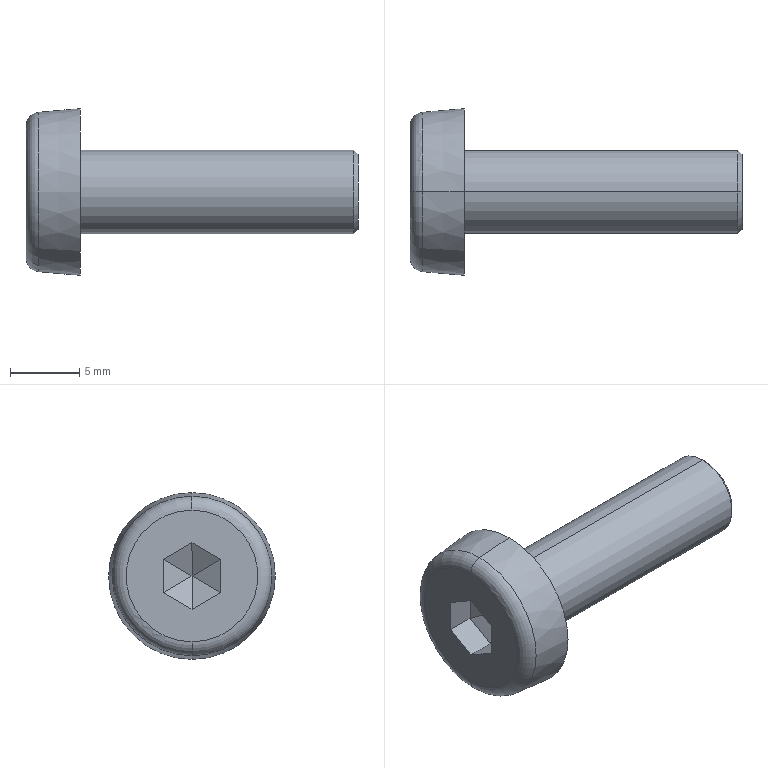Part | SolidWorks | features Cut 2, Fillet 2, Boss 1, Chamfer 1, Extrusion 1, LPattern 1, RevCut 1 | 1 solid | 23 faces | box 23.9 x 12 x 12 mm | volume 939.348 mm3 | plane 15 | cone 4 | torus 2 | cylinder 2 | commonest cylinder face diameters 6 x2
STEP:
#1=CARTESIAN_POINT('',(23.9,0.,-2.7));
#2=VERTEX_POINT('',#1);
#3=CARTESIAN_POINT('',(23.9,0.,2.7));
#4=VERTEX_POINT('',#3);
#5=CARTESIAN_POINT('',(23.9,0.,0.));
#6=DIRECTION('',(1.,0.,0.));
#7=DIRECTION('',(0.,0.,-1.));
#8=AXIS2_PLACEMENT_3D('',#5,#6,#7);
#9=CIRCLE('',#8,2.7);
#10=EDGE_CURVE('',#2,#4,#9,.T.);
#11=ORIENTED_EDGE('',*,*,#10,.F.);
#12=CARTESIAN_POINT('',(23.6,0.,-3.));
#13=VERTEX_POINT('',#12);
#14=CARTESIAN_POINT('',(23.9,0.,-2.7));
#15=DIRECTION('',(-0.7071,0.,-0.7071));
#16=VECTOR('',#15,1000.);
#17=LINE('',#14,#16);
#18=EDGE_CURVE('',#2,#13,#17,.T.);
#19=ORIENTED_EDGE('',*,*,#18,.T.);
#20=CARTESIAN_POINT('',(23.6,0.,3.));
#21=VERTEX_POINT('',#20);
#22=CARTESIAN_POINT('',(23.6,0.,0.));
#23=DIRECTION('',(-1.,0.,0.));
#24=DIRECTION('',(0.,0.,-1.));
#25=AXIS2_PLACEMENT_3D('',#22,#23,#24);
#26=CIRCLE('',#25,3.);
#27=EDGE_CURVE('',#21,#13,#26,.T.);
#28=ORIENTED_EDGE('',*,*,#27,.F.);
#29=CARTESIAN_POINT('',(23.9,0.,2.7));
#30=DIRECTION('',(-0.7071,0.,0.7071));
#31=VECTOR('',#30,1000.);
#32=LINE('',#29,#31);
#33=EDGE_CURVE('',#4,#21,#32,.T.);
#34=ORIENTED_EDGE('',*,*,#33,.F.);
#35=EDGE_LOOP('',(#11,#19,#28,#34));
#36=FACE_OUTER_BOUND('',#35,.T.);
#37=CARTESIAN_POINT('',(23.9,0.,0.));
#38=DIRECTION('',(-1.,0.,0.));
#39=DIRECTION('',(0.,0.,1.));
#40=AXIS2_PLACEMENT_3D('',#37,#38,#39);
#41=CONICAL_SURFACE('',#40,2.7,0.7854);
#42=ADVANCED_FACE('',(#36),#41,.T.);
#43=CARTESIAN_POINT('',(0.,0.,4.742));
#44=VERTEX_POINT('',#43);
#45=CARTESIAN_POINT('',(0.,0.,-4.742));
#46=VERTEX_POINT('',#45);
#47=CARTESIAN_POINT('',(0.,0.,0.));
#48=DIRECTION('',(-1.,0.,0.));
#49=DIRECTION('',(0.,0.,-1.));
#50=AXIS2_PLACEMENT_3D('',#47,#48,#49);
#51=CIRCLE('',#50,4.742);
#52=EDGE_CURVE('',#44,#46,#51,.T.);
#53=ORIENTED_EDGE('',*,*,#52,.F.);
#54=CARTESIAN_POINT('',(0.9128,0.,5.739));
#55=VERTEX_POINT('',#54);
#56=CARTESIAN_POINT('',(1.,0.,4.742));
#57=DIRECTION('',(0.,1.,0.));
#58=DIRECTION('',(0.,0.,1.));
#59=AXIS2_PLACEMENT_3D('',#56,#57,#58);
#60=CIRCLE('',#59,1.);
#61=EDGE_CURVE('',#44,#55,#60,.T.);
#62=ORIENTED_EDGE('',*,*,#61,.T.);
#63=CARTESIAN_POINT('',(0.9128,0.,-5.739));
#64=VERTEX_POINT('',#63);
#65=CARTESIAN_POINT('',(0.9128,0.,0.));
#66=DIRECTION('',(1.,0.,0.));
#67=DIRECTION('',(0.,0.,-1.));
#68=AXIS2_PLACEMENT_3D('',#65,#66,#67);
#69=CIRCLE('',#68,5.739);
#70=EDGE_CURVE('',#64,#55,#69,.T.);
#71=ORIENTED_EDGE('',*,*,#70,.F.);
#72=CARTESIAN_POINT('',(1.,0.,-4.742));
#73=DIRECTION('',(0.,-1.,0.));
#74=DIRECTION('',(0.,0.,-1.));
#75=AXIS2_PLACEMENT_3D('',#72,#73,#74);
#76=CIRCLE('',#75,1.);
#77=EDGE_CURVE('',#46,#64,#76,.T.);
#78=ORIENTED_EDGE('',*,*,#77,.F.);
#79=EDGE_LOOP('',(#53,#62,#71,#78));
#80=FACE_OUTER_BOUND('',#79,.T.);
#81=CARTESIAN_POINT('',(1.,0.,0.));
#82=DIRECTION('',(1.,0.,0.));
#83=DIRECTION('',(0.,0.,-1.));
#84=AXIS2_PLACEMENT_3D('',#81,#82,#83);
#85=TOROIDAL_SURFACE('',#84,4.742,1.);
#86=ADVANCED_FACE('',(#80),#85,.T.);
#87=ORIENTED_EDGE('',*,*,#27,.T.);
#88=CARTESIAN_POINT('',(3.9,0.,-3.));
#89=VERTEX_POINT('',#88);
#90=CARTESIAN_POINT('',(23.9,0.,-3.));
#91=DIRECTION('',(-1.,0.,0.));
#92=VECTOR('',#91,1000.);
#93=LINE('',#90,#92);
#94=EDGE_CURVE('',#13,#89,#93,.T.);
#95=ORIENTED_EDGE('',*,*,#94,.T.);
#96=CARTESIAN_POINT('',(3.9,0.,3.));
#97=VERTEX_POINT('',#96);
#98=CARTESIAN_POINT('',(3.9,0.,0.));
#99=DIRECTION('',(1.,0.,0.));
#100=DIRECTION('',(0.,0.,-1.));
#101=AXIS2_PLACEMENT_3D('',#98,#99,#100);
#102=CIRCLE('',#101,3.);
#103=EDGE_CURVE('',#89,#97,#102,.T.);
#104=ORIENTED_EDGE('',*,*,#103,.T.);
#105=CARTESIAN_POINT('',(23.9,0.,3.));
#106=DIRECTION('',(-1.,0.,0.));
#107=VECTOR('',#106,1000.);
#108=LINE('',#105,#107);
#109=EDGE_CURVE('',#21,#97,#108,.T.);
#110=ORIENTED_EDGE('',*,*,#109,.F.);
#111=EDGE_LOOP('',(#87,#95,#104,#110));
#112=FACE_OUTER_BOUND('',#111,.T.);
#113=CARTESIAN_POINT('',(23.9,0.,0.));
#114=DIRECTION('',(-1.,0.,0.));
#115=DIRECTION('',(0.,0.,1.));
#116=AXIS2_PLACEMENT_3D('',#113,#114,#115);
#117=CYLINDRICAL_SURFACE('',#116,3.);
#118=ADVANCED_FACE('',(#112),#117,.T.);
#119=ORIENTED_EDGE('',*,*,#70,.T.);
#120=CARTESIAN_POINT('',(3.9,0.,6.));
#121=VERTEX_POINT('',#120);
#122=CARTESIAN_POINT('',(3.9,0.,6.));
#123=DIRECTION('',(0.9962,0.,0.08716));
#124=VECTOR('',#123,1000.);
#125=LINE('',#122,#124);
#126=EDGE_CURVE('',#55,#121,#125,.T.);
#127=ORIENTED_EDGE('',*,*,#126,.T.);
#128=CARTESIAN_POINT('',(3.9,0.,-6.));
#129=VERTEX_POINT('',#128);
#130=CARTESIAN_POINT('',(3.9,0.,0.));
#131=DIRECTION('',(1.,0.,0.));
#132=DIRECTION('',(0.,0.,-1.));
#133=AXIS2_PLACEMENT_3D('',#130,#131,#132);
#134=CIRCLE('',#133,6.);
#135=EDGE_CURVE('',#129,#121,#134,.T.);
#136=ORIENTED_EDGE('',*,*,#135,.F.);
#137=CARTESIAN_POINT('',(3.9,0.,-6.));
#138=DIRECTION('',(0.9962,0.,-0.08716));
#139=VECTOR('',#138,1000.);
#140=LINE('',#137,#139);
#141=EDGE_CURVE('',#64,#129,#140,.T.);
#142=ORIENTED_EDGE('',*,*,#141,.F.);
#143=EDGE_LOOP('',(#119,#127,#136,#142));
#144=FACE_OUTER_BOUND('',#143,.T.);
#145=CARTESIAN_POINT('',(3.9,0.,0.));
#146=DIRECTION('',(1.,0.,0.));
#147=DIRECTION('',(0.,0.,-1.));
#148=AXIS2_PLACEMENT_3D('',#145,#146,#147);
#149=CONICAL_SURFACE('',#148,6.,0.08727);
#150=ADVANCED_FACE('',(#144),#149,.T.);
#151=CARTESIAN_POINT('',(0.,0.,0.));
#152=DIRECTION('',(-1.,0.,0.));
#153=DIRECTION('',(0.,0.,-1.));
#154=AXIS2_PLACEMENT_3D('',#151,#152,#153);
#155=CIRCLE('',#154,4.742);
#156=EDGE_CURVE('',#46,#44,#155,.T.);
#157=ORIENTED_EDGE('',*,*,#156,.T.);
#158=ORIENTED_EDGE('',*,*,#52,.T.);
#159=EDGE_LOOP('',(#157,#158));
#160=FACE_OUTER_BOUND('',#159,.T.);
#161=CARTESIAN_POINT('',(0.,-2.075,-1.198));
#162=VERTEX_POINT('',#161);
#163=CARTESIAN_POINT('',(0.,0.,-2.396));
#164=VERTEX_POINT('',#163);
#165=CARTESIAN_POINT('',(0.,-2.075,-1.198));
#166=DIRECTION('',(0.,0.866,-0.5));
#167=VECTOR('',#166,1000.);
#168=LINE('',#165,#167);
#169=EDGE_CURVE('',#162,#164,#168,.T.);
#170=ORIENTED_EDGE('',*,*,#169,.T.);
#171=CARTESIAN_POINT('',(0.,2.075,-1.198));
#172=VERTEX_POINT('',#171);
#173=CARTESIAN_POINT('',(0.,0.,-2.396));
#174=DIRECTION('',(0.,0.866,0.5));
#175=VECTOR('',#174,1000.);
#176=LINE('',#173,#175);
#177=EDGE_CURVE('',#164,#172,#176,.T.);
#178=ORIENTED_EDGE('',*,*,#177,.T.);
#179=CARTESIAN_POINT('',(0.,2.075,1.198));
#180=VERTEX_POINT('',#179);
#181=CARTESIAN_POINT('',(0.,2.075,-1.198));
#182=DIRECTION('',(0.,0.,1.));
#183=VECTOR('',#182,1000.);
#184=LINE('',#181,#183);
#185=EDGE_CURVE('',#172,#180,#184,.T.);
#186=ORIENTED_EDGE('',*,*,#185,.T.);
#187=CARTESIAN_POINT('',(0.,0.,2.396));
#188=VERTEX_POINT('',#187);
#189=CARTESIAN_POINT('',(0.,2.075,1.198));
#190=DIRECTION('',(0.,-0.866,0.5));
#191=VECTOR('',#190,1000.);
#192=LINE('',#189,#191);
#193=EDGE_CURVE('',#180,#188,#192,.T.);
#194=ORIENTED_EDGE('',*,*,#193,.T.);
#195=CARTESIAN_POINT('',(0.,-2.075,1.198));
#196=VERTEX_POINT('',#195);
#197=CARTESIAN_POINT('',(0.,0.,2.396));
#198=DIRECTION('',(0.,-0.866,-0.5));
#199=VECTOR('',#198,1000.);
#200=LINE('',#197,#199);
#201=EDGE_CURVE('',#188,#196,#200,.T.);
#202=ORIENTED_EDGE('',*,*,#201,.T.);
#203=CARTESIAN_POINT('',(0.,-2.075,1.198));
#204=DIRECTION('',(0.,0.,-1.));
#205=VECTOR('',#204,1000.);
#206=LINE('',#203,#205);
#207=EDGE_CURVE('',#196,#162,#206,.T.);
#208=ORIENTED_EDGE('',*,*,#207,.T.);
#209=EDGE_LOOP('',(#170,#178,#186,#194,#202,#208));
#210=FACE_BOUND('',#209,.T.);
#211=CARTESIAN_POINT('',(0.,0.,0.));
#212=DIRECTION('',(1.,0.,0.));
#213=DIRECTION('',(0.,0.,-1.));
#214=AXIS2_PLACEMENT_3D('',#211,#212,#213);
#215=PLANE('',#214);
#216=ADVANCED_FACE('',(#160,#210),#215,.F.);
#217=ORIENTED_EDGE('',*,*,#135,.T.);
#218=CARTESIAN_POINT('',(3.9,0.,0.));
#219=DIRECTION('',(1.,0.,0.));
#220=DIRECTION('',(0.,0.,-1.));
#221=AXIS2_PLACEMENT_3D('',#218,#219,#220);
#222=CIRCLE('',#221,6.);
#223=EDGE_CURVE('',#121,#129,#222,.T.);
#224=ORIENTED_EDGE('',*,*,#223,.T.);
#225=EDGE_LOOP('',(#217,#224));
#226=FACE_OUTER_BOUND('',#225,.T.);
#227=CARTESIAN_POINT('',(3.9,0.,0.));
#228=DIRECTION('',(1.,0.,0.));
#229=DIRECTION('',(0.,0.,-1.));
#230=AXIS2_PLACEMENT_3D('',#227,#228,#229);
#231=CIRCLE('',#230,3.);
#232=EDGE_CURVE('',#97,#89,#231,.T.);
#233=ORIENTED_EDGE('',*,*,#232,.F.);
#234=ORIENTED_EDGE('',*,*,#103,.F.);
#235=EDGE_LOOP('',(#233,#234));
#236=FACE_BOUND('',#235,.T.);
#237=CARTESIAN_POINT('',(3.9,0.,0.));
#238=DIRECTION('',(1.,0.,0.));
#239=DIRECTION('',(0.,0.,-1.));
#240=AXIS2_PLACEMENT_3D('',#237,#238,#239);
#241=PLANE('',#240);
#242=ADVANCED_FACE('',(#226,#236),#241,.T.);
#243=ORIENTED_EDGE('',*,*,#126,.F.);
#244=CARTESIAN_POINT('',(0.9128,0.,0.));
#245=DIRECTION('',(1.,0.,0.));
#246=DIRECTION('',(0.,0.,-1.));
#247=AXIS2_PLACEMENT_3D('',#244,#245,#246);
#248=CIRCLE('',#247,5.739);
#249=EDGE_CURVE('',#55,#64,#248,.T.);
#250=ORIENTED_EDGE('',*,*,#249,.T.);
#251=ORIENTED_EDGE('',*,*,#141,.T.);
#252=ORIENTED_EDGE('',*,*,#223,.F.);
#253=EDGE_LOOP('',(#243,#250,#251,#252));
#254=FACE_OUTER_BOUND('',#253,.T.);
#255=CARTESIAN_POINT('',(3.9,0.,0.));
#256=DIRECTION('',(1.,0.,0.));
#257=DIRECTION('',(0.,0.,-1.));
#258=AXIS2_PLACEMENT_3D('',#255,#256,#257);
#259=CONICAL_SURFACE('',#258,6.,0.08727);
#260=ADVANCED_FACE('',(#254),#259,.T.);
#261=ORIENTED_EDGE('',*,*,#94,.F.);
#262=CARTESIAN_POINT('',(23.6,0.,0.));
#263=DIRECTION('',(-1.,0.,0.));
#264=DIRECTION('',(0.,0.,-1.));
#265=AXIS2_PLACEMENT_3D('',#262,#263,#264);
#266=CIRCLE('',#265,3.);
#267=EDGE_CURVE('',#13,#21,#266,.T.);
#268=ORIENTED_EDGE('',*,*,#267,.T.);
#269=ORIENTED_EDGE('',*,*,#109,.T.);
#270=ORIENTED_EDGE('',*,*,#232,.T.);
#271=EDGE_LOOP('',(#261,#268,#269,#270));
#272=FACE_OUTER_BOUND('',#271,.T.);
#273=CARTESIAN_POINT('',(23.9,0.,0.));
#274=DIRECTION('',(-1.,0.,0.));
#275=DIRECTION('',(0.,0.,1.));
#276=AXIS2_PLACEMENT_3D('',#273,#274,#275);
#277=CYLINDRICAL_SURFACE('',#276,3.);
#278=ADVANCED_FACE('',(#272),#277,.T.);
#279=CARTESIAN_POINT('',(23.9,0.,0.));
#280=DIRECTION('',(1.,0.,0.));
#281=DIRECTION('',(0.,0.,-1.));
#282=AXIS2_PLACEMENT_3D('',#279,#280,#281);
#283=CIRCLE('',#282,2.7);
#284=EDGE_CURVE('',#4,#2,#283,.T.);
#285=ORIENTED_EDGE('',*,*,#284,.T.);
#286=ORIENTED_EDGE('',*,*,#10,.T.);
#287=EDGE_LOOP('',(#285,#286));
#288=FACE_OUTER_BOUND('',#287,.T.);
#289=CARTESIAN_POINT('',(23.9,0.,0.));
#290=DIRECTION('',(1.,0.,0.));
#291=DIRECTION('',(0.,0.,-1.));
#292=AXIS2_PLACEMENT_3D('',#289,#290,#291);
#293=PLANE('',#292);
#294=ADVANCED_FACE('',(#288),#293,.T.);
#295=ORIENTED_EDGE('',*,*,#169,.F.);
#296=CARTESIAN_POINT('',(2.,-2.075,-1.198));
#297=VERTEX_POINT('',#296);
#298=CARTESIAN_POINT('',(2.,-2.075,-1.198));
#299=DIRECTION('',(-1.,0.,0.));
#300=VECTOR('',#299,1000.);
#301=LINE('',#298,#300);
#302=EDGE_CURVE('',#297,#162,#301,.T.);
#303=ORIENTED_EDGE('',*,*,#302,.F.);
#304=CARTESIAN_POINT('',(2.,0.,-2.396));
#305=VERTEX_POINT('',#304);
#306=CARTESIAN_POINT('',(2.,-2.075,-1.198));
#307=DIRECTION('',(0.,0.866,-0.5));
#308=VECTOR('',#307,1000.);
#309=LINE('',#306,#308);
#310=EDGE_CURVE('',#297,#305,#309,.T.);
#311=ORIENTED_EDGE('',*,*,#310,.T.);
#312=CARTESIAN_POINT('',(2.,0.,-2.396));
#313=DIRECTION('',(-1.,0.,0.));
#314=VECTOR('',#313,1000.);
#315=LINE('',#312,#314);
#316=EDGE_CURVE('',#305,#164,#315,.T.);
#317=ORIENTED_EDGE('',*,*,#316,.T.);
#318=EDGE_LOOP('',(#295,#303,#311,#317));
#319=FACE_OUTER_BOUND('',#318,.T.);
#320=CARTESIAN_POINT('',(2.,-2.075,-1.198));
#321=DIRECTION('',(0.,0.5,0.866));
#322=DIRECTION('',(0.,-0.866,0.5));
#323=AXIS2_PLACEMENT_3D('',#320,#321,#322);
#324=PLANE('',#323);
#325=ADVANCED_FACE('',(#319),#324,.T.);
#326=ORIENTED_EDGE('',*,*,#177,.F.);
#327=ORIENTED_EDGE('',*,*,#316,.F.);
#328=CARTESIAN_POINT('',(2.,2.075,-1.198));
#329=VERTEX_POINT('',#328);
#330=CARTESIAN_POINT('',(2.,0.,-2.396));
#331=DIRECTION('',(0.,0.866,0.5));
#332=VECTOR('',#331,1000.);
#333=LINE('',#330,#332);
#334=EDGE_CURVE('',#305,#329,#333,.T.);
#335=ORIENTED_EDGE('',*,*,#334,.T.);
#336=CARTESIAN_POINT('',(2.,2.075,-1.198));
#337=DIRECTION('',(-1.,0.,0.));
#338=VECTOR('',#337,1000.);
#339=LINE('',#336,#338);
#340=EDGE_CURVE('',#329,#172,#339,.T.);
#341=ORIENTED_EDGE('',*,*,#340,.T.);
#342=EDGE_LOOP('',(#326,#327,#335,#341));
#343=FACE_OUTER_BOUND('',#342,.T.);
#344=CARTESIAN_POINT('',(2.,0.,-2.396));
#345=DIRECTION('',(0.,-0.5,0.866));
#346=DIRECTION('',(0.,-0.866,-0.5));
#347=AXIS2_PLACEMENT_3D('',#344,#345,#346);
#348=PLANE('',#347);
#349=ADVANCED_FACE('',(#343),#348,.T.);
#350=ORIENTED_EDGE('',*,*,#185,.F.);
#351=ORIENTED_EDGE('',*,*,#340,.F.);
#352=CARTESIAN_POINT('',(2.,2.075,1.198));
#353=VERTEX_POINT('',#352);
#354=CARTESIAN_POINT('',(2.,2.075,-1.198));
#355=DIRECTION('',(0.,0.,1.));
#356=VECTOR('',#355,1000.);
#357=LINE('',#354,#356);
#358=EDGE_CURVE('',#329,#353,#357,.T.);
#359=ORIENTED_EDGE('',*,*,#358,.T.);
#360=CARTESIAN_POINT('',(2.,2.075,1.198));
#361=DIRECTION('',(-1.,0.,0.));
#362=VECTOR('',#361,1000.);
#363=LINE('',#360,#362);
#364=EDGE_CURVE('',#353,#180,#363,.T.);
#365=ORIENTED_EDGE('',*,*,#364,.T.);
#366=EDGE_LOOP('',(#350,#351,#359,#365));
#367=FACE_OUTER_BOUND('',#366,.T.);
#368=CARTESIAN_POINT('',(2.,2.075,-1.198));
#369=DIRECTION('',(0.,-1.,0.));
#370=DIRECTION('',(0.,0.,-1.));
#371=AXIS2_PLACEMENT_3D('',#368,#369,#370);
#372=PLANE('',#371);
#373=ADVANCED_FACE('',(#367),#372,.T.);
#374=ORIENTED_EDGE('',*,*,#193,.F.);
#375=ORIENTED_EDGE('',*,*,#364,.F.);
#376=CARTESIAN_POINT('',(2.,0.,2.396));
#377=VERTEX_POINT('',#376);
#378=CARTESIAN_POINT('',(2.,2.075,1.198));
#379=DIRECTION('',(0.,-0.866,0.5));
#380=VECTOR('',#379,1000.);
#381=LINE('',#378,#380);
#382=EDGE_CURVE('',#353,#377,#381,.T.);
#383=ORIENTED_EDGE('',*,*,#382,.T.);
#384=CARTESIAN_POINT('',(2.,0.,2.396));
#385=DIRECTION('',(-1.,0.,0.));
#386=VECTOR('',#385,1000.);
#387=LINE('',#384,#386);
#388=EDGE_CURVE('',#377,#188,#387,.T.);
#389=ORIENTED_EDGE('',*,*,#388,.T.);
#390=EDGE_LOOP('',(#374,#375,#383,#389));
#391=FACE_OUTER_BOUND('',#390,.T.);
#392=CARTESIAN_POINT('',(2.,2.075,1.198));
#393=DIRECTION('',(0.,-0.5,-0.866));
#394=DIRECTION('',(0.,0.866,-0.5));
#395=AXIS2_PLACEMENT_3D('',#392,#393,#394);
#396=PLANE('',#395);
#397=ADVANCED_FACE('',(#391),#396,.T.);
#398=ORIENTED_EDGE('',*,*,#201,.F.);
#399=ORIENTED_EDGE('',*,*,#388,.F.);
#400=CARTESIAN_POINT('',(2.,-2.075,1.198));
#401=VERTEX_POINT('',#400);
#402=CARTESIAN_POINT('',(2.,0.,2.396));
#403=DIRECTION('',(0.,-0.866,-0.5));
#404=VECTOR('',#403,1000.);
#405=LINE('',#402,#404);
#406=EDGE_CURVE('',#377,#401,#405,.T.);
#407=ORIENTED_EDGE('',*,*,#406,.T.);
#408=CARTESIAN_POINT('',(2.,-2.075,1.198));
#409=DIRECTION('',(-1.,0.,0.));
#410=VECTOR('',#409,1000.);
#411=LINE('',#408,#410);
#412=EDGE_CURVE('',#401,#196,#411,.T.);
#413=ORIENTED_EDGE('',*,*,#412,.T.);
#414=EDGE_LOOP('',(#398,#399,#407,#413));
#415=FACE_OUTER_BOUND('',#414,.T.);
#416=CARTESIAN_POINT('',(2.,0.,2.396));
#417=DIRECTION('',(0.,0.5,-0.866));
#418=DIRECTION('',(0.,0.866,0.5));
#419=AXIS2_PLACEMENT_3D('',#416,#417,#418);
#420=PLANE('',#419);
#421=ADVANCED_FACE('',(#415),#420,.T.);
#422=ORIENTED_EDGE('',*,*,#207,.F.);
#423=ORIENTED_EDGE('',*,*,#412,.F.);
#424=CARTESIAN_POINT('',(2.,-2.075,1.198));
#425=DIRECTION('',(0.,0.,-1.));
#426=VECTOR('',#425,1000.);
#427=LINE('',#424,#426);
#428=EDGE_CURVE('',#401,#297,#427,.T.);
#429=ORIENTED_EDGE('',*,*,#428,.T.);
#430=ORIENTED_EDGE('',*,*,#302,.T.);
#431=EDGE_LOOP('',(#422,#423,#429,#430));
#432=FACE_OUTER_BOUND('',#431,.T.);
#433=CARTESIAN_POINT('',(2.,-2.075,1.198));
#434=DIRECTION('',(0.,1.,0.));
#435=DIRECTION('',(0.,0.,1.));
#436=AXIS2_PLACEMENT_3D('',#433,#434,#435);
#437=PLANE('',#436);
#438=ADVANCED_FACE('',(#432),#437,.T.);
#439=ORIENTED_EDGE('',*,*,#406,.F.);
#440=CARTESIAN_POINT('',(3.198,0.,0.));
#441=VERTEX_POINT('',#440);
#442=CARTESIAN_POINT('',(2.,0.,2.396));
#443=DIRECTION('',(-0.4472,0.,0.8944));
#444=VECTOR('',#443,1000.);
#445=LINE('',#442,#444);
#446=EDGE_CURVE('',#441,#377,#445,.T.);
#447=ORIENTED_EDGE('',*,*,#446,.F.);
#448=CARTESIAN_POINT('',(2.,-2.075,1.198));
#449=DIRECTION('',(-0.4472,-0.7746,0.4472));
#450=VECTOR('',#449,1000.);
#451=LINE('',#448,#450);
#452=EDGE_CURVE('',#441,#401,#451,.T.);
#453=ORIENTED_EDGE('',*,*,#452,.T.);
#454=EDGE_LOOP('',(#439,#447,#453));
#455=FACE_OUTER_BOUND('',#454,.T.);
#456=CARTESIAN_POINT('',(2.,0.,2.396));
#457=DIRECTION('',(0.866,-0.25,0.433));
#458=DIRECTION('',(0.4472,0.,-0.8944));
#459=AXIS2_PLACEMENT_3D('',#456,#457,#458);
#460=PLANE('',#459);
#461=ADVANCED_FACE('',(#455),#460,.F.);
#462=ORIENTED_EDGE('',*,*,#428,.F.);
#463=ORIENTED_EDGE('',*,*,#452,.F.);
#464=CARTESIAN_POINT('',(2.,-2.075,-1.198));
#465=DIRECTION('',(-0.4472,-0.7746,-0.4472));
#466=VECTOR('',#465,1000.);
#467=LINE('',#464,#466);
#468=EDGE_CURVE('',#441,#297,#467,.T.);
#469=ORIENTED_EDGE('',*,*,#468,.T.);
#470=EDGE_LOOP('',(#462,#463,#469));
#471=FACE_OUTER_BOUND('',#470,.T.);
#472=CARTESIAN_POINT('',(2.,-2.075,1.198));
#473=DIRECTION('',(0.866,-0.5,0.));
#474=DIRECTION('',(0.5,0.866,0.));
#475=AXIS2_PLACEMENT_3D('',#472,#473,#474);
#476=PLANE('',#475);
#477=ADVANCED_FACE('',(#471),#476,.F.);
#478=ORIENTED_EDGE('',*,*,#310,.F.);
#479=ORIENTED_EDGE('',*,*,#468,.F.);
#480=CARTESIAN_POINT('',(2.,0.,-2.396));
#481=DIRECTION('',(-0.4472,0.,-0.8944));
#482=VECTOR('',#481,1000.);
#483=LINE('',#480,#482);
#484=EDGE_CURVE('',#441,#305,#483,.T.);
#485=ORIENTED_EDGE('',*,*,#484,.T.);
#486=EDGE_LOOP('',(#478,#479,#485));
#487=FACE_OUTER_BOUND('',#486,.T.);
#488=CARTESIAN_POINT('',(2.,-2.075,-1.198));
#489=DIRECTION('',(0.866,-0.25,-0.433));
#490=DIRECTION('',(-0.4472,0.,-0.8944));
#491=AXIS2_PLACEMENT_3D('',#488,#489,#490);
#492=PLANE('',#491);
#493=ADVANCED_FACE('',(#487),#492,.F.);
#494=ORIENTED_EDGE('',*,*,#334,.F.);
#495=ORIENTED_EDGE('',*,*,#484,.F.);
#496=CARTESIAN_POINT('',(2.,2.075,-1.198));
#497=DIRECTION('',(-0.4472,0.7746,-0.4472));
#498=VECTOR('',#497,1000.);
#499=LINE('',#496,#498);
#500=EDGE_CURVE('',#441,#329,#499,.T.);
#501=ORIENTED_EDGE('',*,*,#500,.T.);
#502=EDGE_LOOP('',(#494,#495,#501));
#503=FACE_OUTER_BOUND('',#502,.T.);
#504=CARTESIAN_POINT('',(2.,0.,-2.396));
#505=DIRECTION('',(0.866,0.25,-0.433));
#506=DIRECTION('',(-0.4472,0.,-0.8944));
#507=AXIS2_PLACEMENT_3D('',#504,#505,#506);
#508=PLANE('',#507);
#509=ADVANCED_FACE('',(#503),#508,.F.);
#510=ORIENTED_EDGE('',*,*,#358,.F.);
#511=ORIENTED_EDGE('',*,*,#500,.F.);
#512=CARTESIAN_POINT('',(2.,2.075,1.198));
#513=DIRECTION('',(-0.4472,0.7746,0.4472));
#514=VECTOR('',#513,1000.);
#515=LINE('',#512,#514);
#516=EDGE_CURVE('',#441,#353,#515,.T.);
#517=ORIENTED_EDGE('',*,*,#516,.T.);
#518=EDGE_LOOP('',(#510,#511,#517));
#519=FACE_OUTER_BOUND('',#518,.T.);
#520=CARTESIAN_POINT('',(2.,2.075,-1.198));
#521=DIRECTION('',(0.866,0.5,0.));
#522=DIRECTION('',(-0.5,0.866,0.));
#523=AXIS2_PLACEMENT_3D('',#520,#521,#522);
#524=PLANE('',#523);
#525=ADVANCED_FACE('',(#519),#524,.F.);
#526=ORIENTED_EDGE('',*,*,#382,.F.);
#527=ORIENTED_EDGE('',*,*,#516,.F.);
#528=ORIENTED_EDGE('',*,*,#446,.T.);
#529=EDGE_LOOP('',(#526,#527,#528));
#530=FACE_OUTER_BOUND('',#529,.T.);
#531=CARTESIAN_POINT('',(2.,2.075,1.198));
#532=DIRECTION('',(0.866,0.25,0.433));
#533=DIRECTION('',(0.4472,0.,-0.8944));
#534=AXIS2_PLACEMENT_3D('',#531,#532,#533);
#535=PLANE('',#534);
#536=ADVANCED_FACE('',(#530),#535,.F.);
#537=ORIENTED_EDGE('',*,*,#61,.F.);
#538=ORIENTED_EDGE('',*,*,#156,.F.);
#539=ORIENTED_EDGE('',*,*,#77,.T.);
#540=ORIENTED_EDGE('',*,*,#249,.F.);
#541=EDGE_LOOP('',(#537,#538,#539,#540));
#542=FACE_OUTER_BOUND('',#541,.T.);
#543=CARTESIAN_POINT('',(1.,0.,0.));
#544=DIRECTION('',(1.,0.,0.));
#545=DIRECTION('',(0.,0.,-1.));
#546=AXIS2_PLACEMENT_3D('',#543,#544,#545);
#547=TOROIDAL_SURFACE('',#546,4.742,1.);
#548=ADVANCED_FACE('',(#542),#547,.T.);
#549=ORIENTED_EDGE('',*,*,#18,.F.);
#550=ORIENTED_EDGE('',*,*,#284,.F.);
#551=ORIENTED_EDGE('',*,*,#33,.T.);
#552=ORIENTED_EDGE('',*,*,#267,.F.);
#553=EDGE_LOOP('',(#549,#550,#551,#552));
#554=FACE_OUTER_BOUND('',#553,.T.);
#555=CARTESIAN_POINT('',(23.9,0.,0.));
#556=DIRECTION('',(-1.,0.,0.));
#557=DIRECTION('',(0.,0.,1.));
#558=AXIS2_PLACEMENT_3D('',#555,#556,#557);
#559=CONICAL_SURFACE('',#558,2.7,0.7854);
#560=ADVANCED_FACE('',(#554),#559,.T.);
#561=CLOSED_SHELL('',(#42,#86,#118,#150,#216,#242,#260,#278,#294,#325,#349,#373,#397,#421,#438,#461,#477,#493,#509,#525,#536,#548,#560));
#562=MANIFOLD_SOLID_BREP('',#561);
#563=CARTESIAN_POINT('',(0.,0.,0.));
#564=DIRECTION('',(0.,0.,1.));
#565=DIRECTION('',(1.,0.,0.));
#566=AXIS2_PLACEMENT_3D('',#563,#564,#565);
#567=(LENGTH_UNIT()NAMED_UNIT(*)SI_UNIT(.MILLI.,.METRE.));
#568=UNCERTAINTY_MEASURE_WITH_UNIT(LENGTH_MEASURE(0.00001),#567,'','');
#569=(NAMED_UNIT(*)PLANE_ANGLE_UNIT()SI_UNIT($,.RADIAN.));
#570=(NAMED_UNIT(*)SI_UNIT($,.STERADIAN.)SOLID_ANGLE_UNIT());
#571=(GEOMETRIC_REPRESENTATION_CONTEXT(3)GLOBAL_UNCERTAINTY_ASSIGNED_CONTEXT((#568))GLOBAL_UNIT_ASSIGNED_CONTEXT((#567,#569,#570))REPRESENTATION_CONTEXT('',''));
#572=ADVANCED_BREP_SHAPE_REPRESENTATION('',(#562,#566),#571);